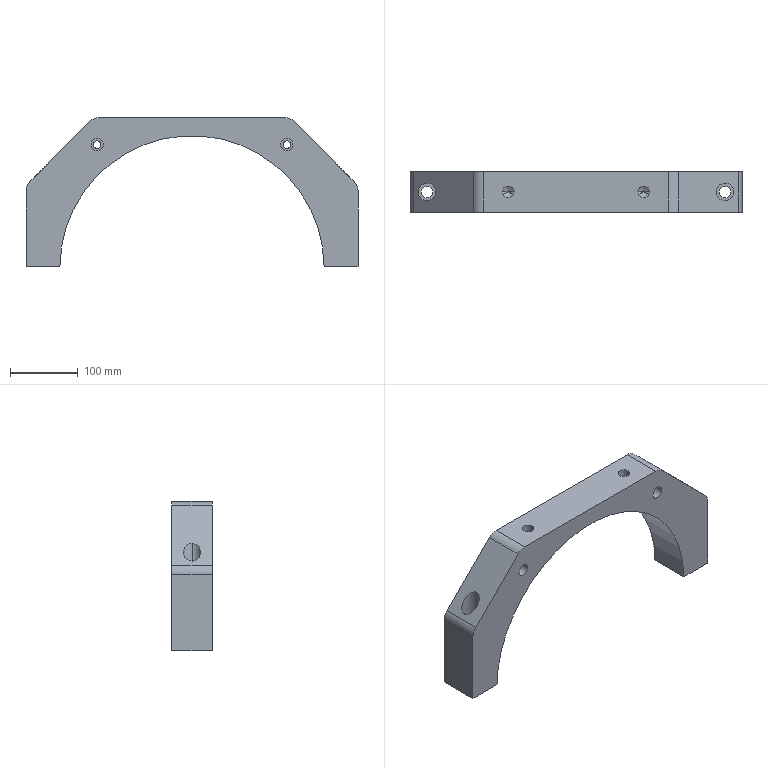Part | NX | features BREP 1 | 1 solid | 48 faces | box 490 x 60 x 220 mm | volume 2146517 mm3 | cylinder 29 | plane 15 | cone 4 | commonest cylinder face diameters 11 x4 17 x4 17.294 x4 18 x4 26 x4 30 x4
STEP:
#1=CARTESIAN_POINT('',(245.,30.,0.));
#2=VERTEX_POINT('',#1);
#3=CARTESIAN_POINT('',(245.,-30.,0.));
#4=VERTEX_POINT('',#3);
#5=CARTESIAN_POINT('',(245.,30.,0.));
#6=DIRECTION('',(0.,-1.,0.));
#7=VECTOR('',#6,1000.);
#8=LINE('',#5,#7);
#9=EDGE_CURVE('',#2,#4,#8,.T.);
#10=ORIENTED_EDGE('',*,*,#9,.F.);
#11=CARTESIAN_POINT('',(245.,30.,111.716));
#12=VERTEX_POINT('',#11);
#13=CARTESIAN_POINT('',(245.,30.,0.));
#14=DIRECTION('',(0.,0.,1.));
#15=VECTOR('',#14,1000.);
#16=LINE('',#13,#15);
#17=EDGE_CURVE('',#2,#12,#16,.T.);
#18=ORIENTED_EDGE('',*,*,#17,.T.);
#19=CARTESIAN_POINT('',(245.,-30.,111.716));
#20=VERTEX_POINT('',#19);
#21=CARTESIAN_POINT('',(245.,-30.,111.716));
#22=DIRECTION('',(0.,1.,0.));
#23=VECTOR('',#22,1000.);
#24=LINE('',#21,#23);
#25=EDGE_CURVE('',#20,#12,#24,.T.);
#26=ORIENTED_EDGE('',*,*,#25,.F.);
#27=CARTESIAN_POINT('',(245.,-30.,0.));
#28=DIRECTION('',(0.,0.,1.));
#29=VECTOR('',#28,1000.);
#30=LINE('',#27,#29);
#31=EDGE_CURVE('',#4,#20,#30,.T.);
#32=ORIENTED_EDGE('',*,*,#31,.F.);
#33=EDGE_LOOP('',(#10,#18,#26,#32));
#34=FACE_BOUND('',#33,.T.);
#35=CARTESIAN_POINT('',(245.,0.,220.));
#36=DIRECTION('',(1.,0.,0.));
#37=DIRECTION('',(0.,1.,0.));
#38=AXIS2_PLACEMENT_3D('',#35,#36,#37);
#39=PLANE('',#38);
#40=ADVANCED_FACE('',(#34),#39,.T.);
#41=CARTESIAN_POINT('',(239.142,-30.,125.858));
#42=VERTEX_POINT('',#41);
#43=CARTESIAN_POINT('',(150.858,-30.,214.142));
#44=VERTEX_POINT('',#43);
#45=CARTESIAN_POINT('',(239.142,-30.,125.858));
#46=DIRECTION('',(-0.7071,0.,0.7071));
#47=VECTOR('',#46,1000.);
#48=LINE('',#45,#47);
#49=EDGE_CURVE('',#42,#44,#48,.T.);
#50=ORIENTED_EDGE('',*,*,#49,.T.);
#51=CARTESIAN_POINT('',(136.716,-30.,220.));
#52=VERTEX_POINT('',#51);
#53=CARTESIAN_POINT('',(136.716,-30.,200.));
#54=DIRECTION('',(0.,-1.,0.));
#55=DIRECTION('',(0.7071,0.,0.7071));
#56=AXIS2_PLACEMENT_3D('',#53,#54,#55);
#57=CIRCLE('',#56,20.);
#58=EDGE_CURVE('',#44,#52,#57,.T.);
#59=ORIENTED_EDGE('',*,*,#58,.T.);
#60=CARTESIAN_POINT('',(-136.716,-30.,220.));
#61=VERTEX_POINT('',#60);
#62=CARTESIAN_POINT('',(136.716,-30.,220.));
#63=DIRECTION('',(-1.,0.,0.));
#64=VECTOR('',#63,1000.);
#65=LINE('',#62,#64);
#66=EDGE_CURVE('',#52,#61,#65,.T.);
#67=ORIENTED_EDGE('',*,*,#66,.T.);
#68=CARTESIAN_POINT('',(-150.858,-30.,214.142));
#69=VERTEX_POINT('',#68);
#70=CARTESIAN_POINT('',(-136.716,-30.,200.));
#71=DIRECTION('',(0.,-1.,0.));
#72=DIRECTION('',(0.,0.,1.));
#73=AXIS2_PLACEMENT_3D('',#70,#71,#72);
#74=CIRCLE('',#73,20.);
#75=EDGE_CURVE('',#61,#69,#74,.T.);
#76=ORIENTED_EDGE('',*,*,#75,.T.);
#77=CARTESIAN_POINT('',(-239.142,-30.,125.858));
#78=VERTEX_POINT('',#77);
#79=CARTESIAN_POINT('',(-150.858,-30.,214.142));
#80=DIRECTION('',(-0.7071,0.,-0.7071));
#81=VECTOR('',#80,1000.);
#82=LINE('',#79,#81);
#83=EDGE_CURVE('',#69,#78,#82,.T.);
#84=ORIENTED_EDGE('',*,*,#83,.T.);
#85=CARTESIAN_POINT('',(-245.,-30.,111.716));
#86=VERTEX_POINT('',#85);
#87=CARTESIAN_POINT('',(-225.,-30.,111.716));
#88=DIRECTION('',(0.,-1.,0.));
#89=DIRECTION('',(-0.7071,0.,0.7071));
#90=AXIS2_PLACEMENT_3D('',#87,#88,#89);
#91=CIRCLE('',#90,20.);
#92=EDGE_CURVE('',#78,#86,#91,.T.);
#93=ORIENTED_EDGE('',*,*,#92,.T.);
#94=CARTESIAN_POINT('',(-245.,-30.,0.));
#95=VERTEX_POINT('',#94);
#96=CARTESIAN_POINT('',(-245.,-30.,111.716));
#97=DIRECTION('',(0.,0.,-1.));
#98=VECTOR('',#97,1000.);
#99=LINE('',#96,#98);
#100=EDGE_CURVE('',#86,#95,#99,.T.);
#101=ORIENTED_EDGE('',*,*,#100,.T.);
#102=CARTESIAN_POINT('',(-194.99,-30.,0.));
#103=VERTEX_POINT('',#102);
#104=CARTESIAN_POINT('',(-245.,-30.,0.));
#105=DIRECTION('',(1.,0.,0.));
#106=VECTOR('',#105,1000.);
#107=LINE('',#104,#106);
#108=EDGE_CURVE('',#95,#103,#107,.T.);
#109=ORIENTED_EDGE('',*,*,#108,.T.);
#110=CARTESIAN_POINT('',(194.99,-30.,0.));
#111=VERTEX_POINT('',#110);
#112=CARTESIAN_POINT('',(0.,-30.,-2.));
#113=DIRECTION('',(0.,1.,0.));
#114=DIRECTION('',(-0.9999,0.,0.01026));
#115=AXIS2_PLACEMENT_3D('',#112,#113,#114);
#116=CIRCLE('',#115,195.);
#117=EDGE_CURVE('',#103,#111,#116,.T.);
#118=ORIENTED_EDGE('',*,*,#117,.T.);
#119=CARTESIAN_POINT('',(194.99,-30.,0.));
#120=DIRECTION('',(1.,0.,0.));
#121=VECTOR('',#120,1000.);
#122=LINE('',#119,#121);
#123=EDGE_CURVE('',#111,#4,#122,.T.);
#124=ORIENTED_EDGE('',*,*,#123,.T.);
#125=ORIENTED_EDGE('',*,*,#31,.T.);
#126=CARTESIAN_POINT('',(225.,-30.,111.716));
#127=DIRECTION('',(0.,-1.,0.));
#128=DIRECTION('',(1.,0.,0.));
#129=AXIS2_PLACEMENT_3D('',#126,#127,#128);
#130=CIRCLE('',#129,20.);
#131=EDGE_CURVE('',#20,#42,#130,.T.);
#132=ORIENTED_EDGE('',*,*,#131,.T.);
#133=EDGE_LOOP('',(#50,#59,#67,#76,#84,#93,#101,#109,#118,#124,#125,#132));
#134=FACE_BOUND('',#133,.T.);
#135=CARTESIAN_POINT('',(131.,-30.,180.));
#136=VERTEX_POINT('',#135);
#137=CARTESIAN_POINT('',(149.,-30.,180.));
#138=VERTEX_POINT('',#137);
#139=CARTESIAN_POINT('',(140.,-30.,180.));
#140=DIRECTION('',(0.,1.,0.));
#141=DIRECTION('',(-1.,0.,0.));
#142=AXIS2_PLACEMENT_3D('',#139,#140,#141);
#143=CIRCLE('',#142,9.);
#144=EDGE_CURVE('',#136,#138,#143,.T.);
#145=ORIENTED_EDGE('',*,*,#144,.T.);
#146=CARTESIAN_POINT('',(140.,-30.,180.));
#147=DIRECTION('',(0.,1.,0.));
#148=DIRECTION('',(1.,0.,0.));
#149=AXIS2_PLACEMENT_3D('',#146,#147,#148);
#150=CIRCLE('',#149,9.);
#151=EDGE_CURVE('',#138,#136,#150,.T.);
#152=ORIENTED_EDGE('',*,*,#151,.T.);
#153=EDGE_LOOP('',(#145,#152));
#154=FACE_BOUND('',#153,.T.);
#155=CARTESIAN_POINT('',(-131.,-30.,180.));
#156=VERTEX_POINT('',#155);
#157=CARTESIAN_POINT('',(-149.,-30.,180.));
#158=VERTEX_POINT('',#157);
#159=CARTESIAN_POINT('',(-140.,-30.,180.));
#160=DIRECTION('',(0.,1.,0.));
#161=DIRECTION('',(1.,0.,0.));
#162=AXIS2_PLACEMENT_3D('',#159,#160,#161);
#163=CIRCLE('',#162,9.);
#164=EDGE_CURVE('',#156,#158,#163,.T.);
#165=ORIENTED_EDGE('',*,*,#164,.T.);
#166=CARTESIAN_POINT('',(-140.,-30.,180.));
#167=DIRECTION('',(0.,1.,0.));
#168=DIRECTION('',(-1.,0.,0.));
#169=AXIS2_PLACEMENT_3D('',#166,#167,#168);
#170=CIRCLE('',#169,9.);
#171=EDGE_CURVE('',#158,#156,#170,.T.);
#172=ORIENTED_EDGE('',*,*,#171,.T.);
#173=EDGE_LOOP('',(#165,#172));
#174=FACE_BOUND('',#173,.T.);
#175=CARTESIAN_POINT('',(0.,-30.,0.));
#176=DIRECTION('',(0.,1.,0.));
#177=DIRECTION('',(1.,0.,0.));
#178=AXIS2_PLACEMENT_3D('',#175,#176,#177);
#179=PLANE('',#178);
#180=ADVANCED_FACE('',(#134,#154,#174),#179,.F.);
#181=CARTESIAN_POINT('',(239.142,30.,125.858));
#182=VERTEX_POINT('',#181);
#183=CARTESIAN_POINT('',(239.142,30.,125.858));
#184=DIRECTION('',(0.,-1.,0.));
#185=VECTOR('',#184,1000.);
#186=LINE('',#183,#185);
#187=EDGE_CURVE('',#182,#42,#186,.T.);
#188=ORIENTED_EDGE('',*,*,#187,.T.);
#189=ORIENTED_EDGE('',*,*,#131,.F.);
#190=ORIENTED_EDGE('',*,*,#25,.T.);
#191=CARTESIAN_POINT('',(225.,30.,111.716));
#192=DIRECTION('',(0.,1.,0.));
#193=DIRECTION('',(0.7071,0.,0.7071));
#194=AXIS2_PLACEMENT_3D('',#191,#192,#193);
#195=CIRCLE('',#194,20.);
#196=EDGE_CURVE('',#182,#12,#195,.T.);
#197=ORIENTED_EDGE('',*,*,#196,.F.);
#198=EDGE_LOOP('',(#188,#189,#190,#197));
#199=FACE_BOUND('',#198,.T.);
#200=CARTESIAN_POINT('',(225.,0.,111.716));
#201=DIRECTION('',(0.,1.,0.));
#202=DIRECTION('',(0.7071,0.,0.7071));
#203=AXIS2_PLACEMENT_3D('',#200,#201,#202);
#204=CYLINDRICAL_SURFACE('',#203,20.);
#205=ADVANCED_FACE('',(#199),#204,.T.);
#206=CARTESIAN_POINT('',(194.99,30.,0.));
#207=VERTEX_POINT('',#206);
#208=CARTESIAN_POINT('',(194.99,30.,0.));
#209=DIRECTION('',(1.,0.,0.));
#210=VECTOR('',#209,1000.);
#211=LINE('',#208,#210);
#212=EDGE_CURVE('',#207,#2,#211,.T.);
#213=ORIENTED_EDGE('',*,*,#212,.F.);
#214=CARTESIAN_POINT('',(-194.99,30.,0.));
#215=VERTEX_POINT('',#214);
#216=CARTESIAN_POINT('',(0.,30.,-2.));
#217=DIRECTION('',(0.,-1.,0.));
#218=DIRECTION('',(0.9999,0.,0.01026));
#219=AXIS2_PLACEMENT_3D('',#216,#217,#218);
#220=CIRCLE('',#219,195.);
#221=EDGE_CURVE('',#207,#215,#220,.T.);
#222=ORIENTED_EDGE('',*,*,#221,.T.);
#223=CARTESIAN_POINT('',(-245.,30.,0.));
#224=VERTEX_POINT('',#223);
#225=CARTESIAN_POINT('',(-245.,30.,0.));
#226=DIRECTION('',(1.,0.,0.));
#227=VECTOR('',#226,1000.);
#228=LINE('',#225,#227);
#229=EDGE_CURVE('',#224,#215,#228,.T.);
#230=ORIENTED_EDGE('',*,*,#229,.F.);
#231=CARTESIAN_POINT('',(-245.,30.,111.716));
#232=VERTEX_POINT('',#231);
#233=CARTESIAN_POINT('',(-245.,30.,111.716));
#234=DIRECTION('',(0.,0.,-1.));
#235=VECTOR('',#234,1000.);
#236=LINE('',#233,#235);
#237=EDGE_CURVE('',#232,#224,#236,.T.);
#238=ORIENTED_EDGE('',*,*,#237,.F.);
#239=CARTESIAN_POINT('',(-239.142,30.,125.858));
#240=VERTEX_POINT('',#239);
#241=CARTESIAN_POINT('',(-225.,30.,111.716));
#242=DIRECTION('',(0.,1.,0.));
#243=DIRECTION('',(-1.,0.,0.));
#244=AXIS2_PLACEMENT_3D('',#241,#242,#243);
#245=CIRCLE('',#244,20.);
#246=EDGE_CURVE('',#232,#240,#245,.T.);
#247=ORIENTED_EDGE('',*,*,#246,.T.);
#248=CARTESIAN_POINT('',(-150.858,30.,214.142));
#249=VERTEX_POINT('',#248);
#250=CARTESIAN_POINT('',(-239.142,30.,125.858));
#251=DIRECTION('',(0.7071,0.,0.7071));
#252=VECTOR('',#251,1000.);
#253=LINE('',#250,#252);
#254=EDGE_CURVE('',#240,#249,#253,.T.);
#255=ORIENTED_EDGE('',*,*,#254,.T.);
#256=CARTESIAN_POINT('',(-136.716,30.,220.));
#257=VERTEX_POINT('',#256);
#258=CARTESIAN_POINT('',(-136.716,30.,200.));
#259=DIRECTION('',(0.,1.,0.));
#260=DIRECTION('',(-0.7071,0.,0.7071));
#261=AXIS2_PLACEMENT_3D('',#258,#259,#260);
#262=CIRCLE('',#261,20.);
#263=EDGE_CURVE('',#249,#257,#262,.T.);
#264=ORIENTED_EDGE('',*,*,#263,.T.);
#265=CARTESIAN_POINT('',(136.716,30.,220.));
#266=VERTEX_POINT('',#265);
#267=CARTESIAN_POINT('',(136.716,30.,220.));
#268=DIRECTION('',(-1.,0.,0.));
#269=VECTOR('',#268,1000.);
#270=LINE('',#267,#269);
#271=EDGE_CURVE('',#266,#257,#270,.T.);
#272=ORIENTED_EDGE('',*,*,#271,.F.);
#273=CARTESIAN_POINT('',(150.858,30.,214.142));
#274=VERTEX_POINT('',#273);
#275=CARTESIAN_POINT('',(136.716,30.,200.));
#276=DIRECTION('',(0.,1.,0.));
#277=DIRECTION('',(0.,0.,1.));
#278=AXIS2_PLACEMENT_3D('',#275,#276,#277);
#279=CIRCLE('',#278,20.);
#280=EDGE_CURVE('',#266,#274,#279,.T.);
#281=ORIENTED_EDGE('',*,*,#280,.T.);
#282=CARTESIAN_POINT('',(150.858,30.,214.142));
#283=DIRECTION('',(0.7071,0.,-0.7071));
#284=VECTOR('',#283,1000.);
#285=LINE('',#282,#284);
#286=EDGE_CURVE('',#274,#182,#285,.T.);
#287=ORIENTED_EDGE('',*,*,#286,.T.);
#288=ORIENTED_EDGE('',*,*,#196,.T.);
#289=ORIENTED_EDGE('',*,*,#17,.F.);
#290=EDGE_LOOP('',(#213,#222,#230,#238,#247,#255,#264,#272,#281,#287,#288,#289));
#291=FACE_BOUND('',#290,.T.);
#292=CARTESIAN_POINT('',(125.,30.,180.));
#293=VERTEX_POINT('',#292);
#294=CARTESIAN_POINT('',(155.,30.,180.));
#295=VERTEX_POINT('',#294);
#296=CARTESIAN_POINT('',(140.,30.,180.));
#297=DIRECTION('',(0.,-1.,0.));
#298=DIRECTION('',(-1.,0.,0.));
#299=AXIS2_PLACEMENT_3D('',#296,#297,#298);
#300=CIRCLE('',#299,15.);
#301=EDGE_CURVE('',#293,#295,#300,.T.);
#302=ORIENTED_EDGE('',*,*,#301,.T.);
#303=CARTESIAN_POINT('',(140.,30.,180.));
#304=DIRECTION('',(0.,-1.,0.));
#305=DIRECTION('',(1.,0.,0.));
#306=AXIS2_PLACEMENT_3D('',#303,#304,#305);
#307=CIRCLE('',#306,15.);
#308=EDGE_CURVE('',#295,#293,#307,.T.);
#309=ORIENTED_EDGE('',*,*,#308,.T.);
#310=EDGE_LOOP('',(#302,#309));
#311=FACE_BOUND('',#310,.T.);
#312=CARTESIAN_POINT('',(-125.,30.,180.));
#313=VERTEX_POINT('',#312);
#314=CARTESIAN_POINT('',(-155.,30.,180.));
#315=VERTEX_POINT('',#314);
#316=CARTESIAN_POINT('',(-140.,30.,180.));
#317=DIRECTION('',(0.,-1.,0.));
#318=DIRECTION('',(1.,0.,0.));
#319=AXIS2_PLACEMENT_3D('',#316,#317,#318);
#320=CIRCLE('',#319,15.);
#321=EDGE_CURVE('',#313,#315,#320,.T.);
#322=ORIENTED_EDGE('',*,*,#321,.T.);
#323=CARTESIAN_POINT('',(-140.,30.,180.));
#324=DIRECTION('',(0.,-1.,0.));
#325=DIRECTION('',(-1.,0.,0.));
#326=AXIS2_PLACEMENT_3D('',#323,#324,#325);
#327=CIRCLE('',#326,15.);
#328=EDGE_CURVE('',#315,#313,#327,.T.);
#329=ORIENTED_EDGE('',*,*,#328,.T.);
#330=EDGE_LOOP('',(#322,#329));
#331=FACE_BOUND('',#330,.T.);
#332=CARTESIAN_POINT('',(0.,30.,0.));
#333=DIRECTION('',(0.,1.,0.));
#334=DIRECTION('',(1.,0.,0.));
#335=AXIS2_PLACEMENT_3D('',#332,#333,#334);
#336=PLANE('',#335);
#337=ADVANCED_FACE('',(#291,#311,#331),#336,.T.);
#338=CARTESIAN_POINT('',(150.858,-30.,214.142));
#339=DIRECTION('',(0.,1.,0.));
#340=VECTOR('',#339,1000.);
#341=LINE('',#338,#340);
#342=EDGE_CURVE('',#44,#274,#341,.T.);
#343=ORIENTED_EDGE('',*,*,#342,.F.);
#344=ORIENTED_EDGE('',*,*,#49,.F.);
#345=ORIENTED_EDGE('',*,*,#187,.F.);
#346=ORIENTED_EDGE('',*,*,#286,.F.);
#347=EDGE_LOOP('',(#343,#344,#345,#346));
#348=FACE_BOUND('',#347,.T.);
#349=CARTESIAN_POINT('',(233.,0.,132.));
#350=VERTEX_POINT('',#349);
#351=CARTESIAN_POINT('',(207.,0.,158.));
#352=VERTEX_POINT('',#351);
#353=CARTESIAN_POINT('',(233.,0.,132.));
#354=CARTESIAN_POINT('',(233.,-0.757,132.));
#355=CARTESIAN_POINT('',(232.865,-2.26,132.135));
#356=CARTESIAN_POINT('',(232.31,-4.393,132.69));
#357=CARTESIAN_POINT('',(231.246,-6.675,133.754));
#358=CARTESIAN_POINT('',(230.126,-8.23,134.874));
#359=CARTESIAN_POINT('',(228.875,-9.533,136.125));
#360=CARTESIAN_POINT('',(227.886,-10.366,137.114));
#361=CARTESIAN_POINT('',(226.8,-11.107,138.2));
#362=CARTESIAN_POINT('',(225.679,-11.722,139.321));
#363=CARTESIAN_POINT('',(224.317,-12.294,140.683));
#364=CARTESIAN_POINT('',(222.526,-12.816,142.474));
#365=CARTESIAN_POINT('',(220.151,-13.102,144.849));
#366=CARTESIAN_POINT('',(217.735,-12.866,147.265));
#367=CARTESIAN_POINT('',(215.917,-12.373,149.083));
#368=CARTESIAN_POINT('',(214.533,-11.822,150.467));
#369=CARTESIAN_POINT('',(213.375,-11.214,151.625));
#370=CARTESIAN_POINT('',(212.257,-10.476,152.743));
#371=CARTESIAN_POINT('',(211.239,-9.64,153.761));
#372=CARTESIAN_POINT('',(209.95,-8.325,155.05));
#373=CARTESIAN_POINT('',(208.797,-6.751,156.203));
#374=CARTESIAN_POINT('',(207.701,-4.432,157.299));
#375=CARTESIAN_POINT('',(207.138,-2.286,157.862));
#376=CARTESIAN_POINT('',(207.,-0.7657,158.));
#377=CARTESIAN_POINT('',(207.,0.,158.));
#378=B_SPLINE_CURVE_WITH_KNOTS('',3,(#353,#354,#355,#356,#357,#358,#359,#360,#361,#362,#363,#364,#365,#366,#367,#368,#369,#370,#371,#372,#373,#374,#375,#376,#377),.UNSPECIFIED.,.F.,.F.,(4,1,1,1,1,1,1,1,1,1,1,1,1,1,1,1,1,1,1,1,1,1,4),(0.,0.0625,0.125,0.1875,0.25,0.2812,0.3125,0.3438,0.375,0.4062,0.4375,0.5,0.5625,0.5938,0.625,0.6562,0.6875,0.7188,0.75,0.8125,0.875,0.9375,1.),.UNSPECIFIED.);
#379=EDGE_CURVE('',#350,#352,#378,.T.);
#380=ORIENTED_EDGE('',*,*,#379,.T.);
#381=CARTESIAN_POINT('',(207.,0.,158.));
#382=CARTESIAN_POINT('',(207.,0.7586,158.));
#383=CARTESIAN_POINT('',(207.136,2.265,157.864));
#384=CARTESIAN_POINT('',(207.693,4.402,157.307));
#385=CARTESIAN_POINT('',(208.762,6.688,156.238));
#386=CARTESIAN_POINT('',(209.885,8.244,155.115));
#387=CARTESIAN_POINT('',(211.142,9.549,153.858));
#388=CARTESIAN_POINT('',(212.135,10.382,152.865));
#389=CARTESIAN_POINT('',(213.226,11.123,151.774));
#390=CARTESIAN_POINT('',(214.352,11.736,150.648));
#391=CARTESIAN_POINT('',(215.717,12.306,149.283));
#392=CARTESIAN_POINT('',(217.512,12.823,147.488));
#393=CARTESIAN_POINT('',(219.895,13.103,145.105));
#394=CARTESIAN_POINT('',(222.304,12.859,142.696));
#395=CARTESIAN_POINT('',(224.118,12.362,140.882));
#396=CARTESIAN_POINT('',(225.5,11.807,139.5));
#397=CARTESIAN_POINT('',(226.652,11.198,138.348));
#398=CARTESIAN_POINT('',(227.764,10.46,137.236));
#399=CARTESIAN_POINT('',(228.778,9.625,136.222));
#400=CARTESIAN_POINT('',(230.061,8.311,134.939));
#401=CARTESIAN_POINT('',(231.207,6.743,133.793));
#402=CARTESIAN_POINT('',(232.299,4.43,132.701));
#403=CARTESIAN_POINT('',(232.862,2.284,132.138));
#404=CARTESIAN_POINT('',(233.,0.765,132.));
#405=CARTESIAN_POINT('',(233.,0.,132.));
#406=B_SPLINE_CURVE_WITH_KNOTS('',3,(#381,#382,#383,#384,#385,#386,#387,#388,#389,#390,#391,#392,#393,#394,#395,#396,#397,#398,#399,#400,#401,#402,#403,#404,#405),.UNSPECIFIED.,.F.,.F.,(4,1,1,1,1,1,1,1,1,1,1,1,1,1,1,1,1,1,1,1,1,1,4),(0.,0.0625,0.125,0.1875,0.25,0.2812,0.3125,0.3438,0.375,0.4062,0.4375,0.5,0.5625,0.5938,0.625,0.6562,0.6875,0.7188,0.75,0.8125,0.875,0.9375,1.),.UNSPECIFIED.);
#407=EDGE_CURVE('',#352,#350,#406,.T.);
#408=ORIENTED_EDGE('',*,*,#407,.T.);
#409=EDGE_LOOP('',(#380,#408));
#410=FACE_BOUND('',#409,.T.);
#411=CARTESIAN_POINT('',(245.,0.,120.));
#412=DIRECTION('',(0.7071,0.,0.7071));
#413=DIRECTION('',(0.,-1.,0.));
#414=AXIS2_PLACEMENT_3D('',#411,#412,#413);
#415=PLANE('',#414);
#416=ADVANCED_FACE('',(#348,#410),#415,.T.);
#417=CARTESIAN_POINT('',(136.716,30.,220.));
#418=DIRECTION('',(0.,-1.,0.));
#419=VECTOR('',#418,1000.);
#420=LINE('',#417,#419);
#421=EDGE_CURVE('',#266,#52,#420,.T.);
#422=ORIENTED_EDGE('',*,*,#421,.T.);
#423=ORIENTED_EDGE('',*,*,#58,.F.);
#424=ORIENTED_EDGE('',*,*,#342,.T.);
#425=ORIENTED_EDGE('',*,*,#280,.F.);
#426=EDGE_LOOP('',(#422,#423,#424,#425));
#427=FACE_BOUND('',#426,.T.);
#428=CARTESIAN_POINT('',(136.716,0.,200.));
#429=DIRECTION('',(0.,1.,0.));
#430=DIRECTION('',(0.,0.,1.));
#431=AXIS2_PLACEMENT_3D('',#428,#429,#430);
#432=CYLINDRICAL_SURFACE('',#431,20.);
#433=ADVANCED_FACE('',(#427),#432,.T.);
#434=ORIENTED_EDGE('',*,*,#271,.T.);
#435=CARTESIAN_POINT('',(-136.716,-30.,220.));
#436=DIRECTION('',(0.,1.,0.));
#437=VECTOR('',#436,1000.);
#438=LINE('',#435,#437);
#439=EDGE_CURVE('',#61,#257,#438,.T.);
#440=ORIENTED_EDGE('',*,*,#439,.F.);
#441=ORIENTED_EDGE('',*,*,#66,.F.);
#442=ORIENTED_EDGE('',*,*,#421,.F.);
#443=EDGE_LOOP('',(#434,#440,#441,#442));
#444=FACE_BOUND('',#443,.T.);
#445=CARTESIAN_POINT('',(-91.353,0.,220.));
#446=VERTEX_POINT('',#445);
#447=CARTESIAN_POINT('',(-108.647,0.,220.));
#448=VERTEX_POINT('',#447);
#449=CARTESIAN_POINT('',(-100.,0.,220.));
#450=DIRECTION('',(0.,0.,-1.));
#451=DIRECTION('',(1.,0.,0.));
#452=AXIS2_PLACEMENT_3D('',#449,#450,#451);
#453=CIRCLE('',#452,8.647);
#454=EDGE_CURVE('',#446,#448,#453,.T.);
#455=ORIENTED_EDGE('',*,*,#454,.T.);
#456=CARTESIAN_POINT('',(-100.,0.,220.));
#457=DIRECTION('',(0.,0.,-1.));
#458=DIRECTION('',(-1.,0.,0.));
#459=AXIS2_PLACEMENT_3D('',#456,#457,#458);
#460=CIRCLE('',#459,8.647);
#461=EDGE_CURVE('',#448,#446,#460,.T.);
#462=ORIENTED_EDGE('',*,*,#461,.T.);
#463=EDGE_LOOP('',(#455,#462));
#464=FACE_BOUND('',#463,.T.);
#465=CARTESIAN_POINT('',(108.647,0.,220.));
#466=VERTEX_POINT('',#465);
#467=CARTESIAN_POINT('',(91.353,0.,220.));
#468=VERTEX_POINT('',#467);
#469=CARTESIAN_POINT('',(100.,0.,220.));
#470=DIRECTION('',(0.,0.,-1.));
#471=DIRECTION('',(1.,0.,0.));
#472=AXIS2_PLACEMENT_3D('',#469,#470,#471);
#473=CIRCLE('',#472,8.647);
#474=EDGE_CURVE('',#466,#468,#473,.T.);
#475=ORIENTED_EDGE('',*,*,#474,.T.);
#476=CARTESIAN_POINT('',(100.,0.,220.));
#477=DIRECTION('',(0.,0.,-1.));
#478=DIRECTION('',(-1.,0.,0.));
#479=AXIS2_PLACEMENT_3D('',#476,#477,#478);
#480=CIRCLE('',#479,8.647);
#481=EDGE_CURVE('',#468,#466,#480,.T.);
#482=ORIENTED_EDGE('',*,*,#481,.T.);
#483=EDGE_LOOP('',(#475,#482));
#484=FACE_BOUND('',#483,.T.);
#485=CARTESIAN_POINT('',(245.,0.,220.));
#486=DIRECTION('',(0.,0.,-1.));
#487=DIRECTION('',(0.,-1.,0.));
#488=AXIS2_PLACEMENT_3D('',#485,#486,#487);
#489=PLANE('',#488);
#490=ADVANCED_FACE('',(#444,#464,#484),#489,.F.);
#491=CARTESIAN_POINT('',(-150.858,30.,214.142));
#492=DIRECTION('',(0.,-1.,0.));
#493=VECTOR('',#492,1000.);
#494=LINE('',#491,#493);
#495=EDGE_CURVE('',#249,#69,#494,.T.);
#496=ORIENTED_EDGE('',*,*,#495,.T.);
#497=ORIENTED_EDGE('',*,*,#75,.F.);
#498=ORIENTED_EDGE('',*,*,#439,.T.);
#499=ORIENTED_EDGE('',*,*,#263,.F.);
#500=EDGE_LOOP('',(#496,#497,#498,#499));
#501=FACE_BOUND('',#500,.T.);
#502=CARTESIAN_POINT('',(-136.716,0.,200.));
#503=DIRECTION('',(0.,1.,0.));
#504=DIRECTION('',(-0.7071,0.,0.7071));
#505=AXIS2_PLACEMENT_3D('',#502,#503,#504);
#506=CYLINDRICAL_SURFACE('',#505,20.);
#507=ADVANCED_FACE('',(#501),#506,.T.);
#508=ORIENTED_EDGE('',*,*,#83,.F.);
#509=ORIENTED_EDGE('',*,*,#495,.F.);
#510=ORIENTED_EDGE('',*,*,#254,.F.);
#511=CARTESIAN_POINT('',(-239.142,-30.,125.858));
#512=DIRECTION('',(0.,1.,0.));
#513=VECTOR('',#512,1000.);
#514=LINE('',#511,#513);
#515=EDGE_CURVE('',#78,#240,#514,.T.);
#516=ORIENTED_EDGE('',*,*,#515,.F.);
#517=EDGE_LOOP('',(#508,#509,#510,#516));
#518=FACE_BOUND('',#517,.T.);
#519=CARTESIAN_POINT('',(-233.,0.,132.));
#520=VERTEX_POINT('',#519);
#521=CARTESIAN_POINT('',(-207.,0.,158.));
#522=VERTEX_POINT('',#521);
#523=CARTESIAN_POINT('',(-233.,0.,132.));
#524=CARTESIAN_POINT('',(-233.,0.757,132.));
#525=CARTESIAN_POINT('',(-232.865,2.26,132.135));
#526=CARTESIAN_POINT('',(-232.31,4.393,132.69));
#527=CARTESIAN_POINT('',(-231.246,6.675,133.754));
#528=CARTESIAN_POINT('',(-230.126,8.23,134.874));
#529=CARTESIAN_POINT('',(-228.875,9.533,136.125));
#530=CARTESIAN_POINT('',(-227.886,10.366,137.114));
#531=CARTESIAN_POINT('',(-226.8,11.107,138.2));
#532=CARTESIAN_POINT('',(-225.679,11.722,139.321));
#533=CARTESIAN_POINT('',(-224.317,12.294,140.683));
#534=CARTESIAN_POINT('',(-222.526,12.816,142.474));
#535=CARTESIAN_POINT('',(-220.151,13.102,144.849));
#536=CARTESIAN_POINT('',(-217.735,12.866,147.265));
#537=CARTESIAN_POINT('',(-215.917,12.373,149.083));
#538=CARTESIAN_POINT('',(-214.533,11.822,150.467));
#539=CARTESIAN_POINT('',(-213.375,11.214,151.625));
#540=CARTESIAN_POINT('',(-212.257,10.476,152.743));
#541=CARTESIAN_POINT('',(-211.239,9.64,153.761));
#542=CARTESIAN_POINT('',(-209.95,8.325,155.05));
#543=CARTESIAN_POINT('',(-208.797,6.751,156.203));
#544=CARTESIAN_POINT('',(-207.701,4.432,157.299));
#545=CARTESIAN_POINT('',(-207.138,2.286,157.862));
#546=CARTESIAN_POINT('',(-207.,0.7657,158.));
#547=CARTESIAN_POINT('',(-207.,0.,158.));
#548=B_SPLINE_CURVE_WITH_KNOTS('',3,(#523,#524,#525,#526,#527,#528,#529,#530,#531,#532,#533,#534,#535,#536,#537,#538,#539,#540,#541,#542,#543,#544,#545,#546,#547),.UNSPECIFIED.,.F.,.F.,(4,1,1,1,1,1,1,1,1,1,1,1,1,1,1,1,1,1,1,1,1,1,4),(0.,0.0625,0.125,0.1875,0.25,0.2812,0.3125,0.3438,0.375,0.4062,0.4375,0.5,0.5625,0.5938,0.625,0.6562,0.6875,0.7188,0.75,0.8125,0.875,0.9375,1.),.UNSPECIFIED.);
#549=EDGE_CURVE('',#520,#522,#548,.T.);
#550=ORIENTED_EDGE('',*,*,#549,.T.);
#551=CARTESIAN_POINT('',(-207.,0.,158.));
#552=CARTESIAN_POINT('',(-207.,-0.7586,158.));
#553=CARTESIAN_POINT('',(-207.136,-2.265,157.864));
#554=CARTESIAN_POINT('',(-207.693,-4.402,157.307));
#555=CARTESIAN_POINT('',(-208.762,-6.688,156.238));
#556=CARTESIAN_POINT('',(-209.885,-8.244,155.115));
#557=CARTESIAN_POINT('',(-211.142,-9.549,153.858));
#558=CARTESIAN_POINT('',(-212.135,-10.382,152.865));
#559=CARTESIAN_POINT('',(-213.226,-11.123,151.774));
#560=CARTESIAN_POINT('',(-214.352,-11.736,150.648));
#561=CARTESIAN_POINT('',(-215.717,-12.306,149.283));
#562=CARTESIAN_POINT('',(-217.512,-12.823,147.488));
#563=CARTESIAN_POINT('',(-219.895,-13.103,145.105));
#564=CARTESIAN_POINT('',(-222.304,-12.859,142.696));
#565=CARTESIAN_POINT('',(-224.118,-12.362,140.882));
#566=CARTESIAN_POINT('',(-225.5,-11.807,139.5));
#567=CARTESIAN_POINT('',(-226.652,-11.198,138.348));
#568=CARTESIAN_POINT('',(-227.764,-10.46,137.236));
#569=CARTESIAN_POINT('',(-228.778,-9.625,136.222));
#570=CARTESIAN_POINT('',(-230.061,-8.311,134.939));
#571=CARTESIAN_POINT('',(-231.207,-6.743,133.793));
#572=CARTESIAN_POINT('',(-232.299,-4.43,132.701));
#573=CARTESIAN_POINT('',(-232.862,-2.284,132.138));
#574=CARTESIAN_POINT('',(-233.,-0.765,132.));
#575=CARTESIAN_POINT('',(-233.,0.,132.));
#576=B_SPLINE_CURVE_WITH_KNOTS('',3,(#551,#552,#553,#554,#555,#556,#557,#558,#559,#560,#561,#562,#563,#564,#565,#566,#567,#568,#569,#570,#571,#572,#573,#574,#575),.UNSPECIFIED.,.F.,.F.,(4,1,1,1,1,1,1,1,1,1,1,1,1,1,1,1,1,1,1,1,1,1,4),(0.,0.0625,0.125,0.1875,0.25,0.2812,0.3125,0.3438,0.375,0.4062,0.4375,0.5,0.5625,0.5938,0.625,0.6562,0.6875,0.7188,0.75,0.8125,0.875,0.9375,1.),.UNSPECIFIED.);
#577=EDGE_CURVE('',#522,#520,#576,.T.);
#578=ORIENTED_EDGE('',*,*,#577,.T.);
#579=EDGE_LOOP('',(#550,#578));
#580=FACE_BOUND('',#579,.T.);
#581=CARTESIAN_POINT('',(-245.,0.,120.));
#582=DIRECTION('',(0.7071,0.,-0.7071));
#583=DIRECTION('',(0.,-1.,0.));
#584=AXIS2_PLACEMENT_3D('',#581,#582,#583);
#585=PLANE('',#584);
#586=ADVANCED_FACE('',(#518,#580),#585,.F.);
#587=CARTESIAN_POINT('',(-245.,30.,111.716));
#588=DIRECTION('',(0.,-1.,0.));
#589=VECTOR('',#588,1000.);
#590=LINE('',#587,#589);
#591=EDGE_CURVE('',#232,#86,#590,.T.);
#592=ORIENTED_EDGE('',*,*,#591,.T.);
#593=ORIENTED_EDGE('',*,*,#92,.F.);
#594=ORIENTED_EDGE('',*,*,#515,.T.);
#595=ORIENTED_EDGE('',*,*,#246,.F.);
#596=EDGE_LOOP('',(#592,#593,#594,#595));
#597=FACE_BOUND('',#596,.T.);
#598=CARTESIAN_POINT('',(-225.,0.,111.716));
#599=DIRECTION('',(0.,1.,0.));
#600=DIRECTION('',(-1.,0.,0.));
#601=AXIS2_PLACEMENT_3D('',#598,#599,#600);
#602=CYLINDRICAL_SURFACE('',#601,20.);
#603=ADVANCED_FACE('',(#597),#602,.T.);
#604=CARTESIAN_POINT('',(-245.,30.,0.));
#605=DIRECTION('',(0.,-1.,0.));
#606=VECTOR('',#605,1000.);
#607=LINE('',#604,#606);
#608=EDGE_CURVE('',#224,#95,#607,.T.);
#609=ORIENTED_EDGE('',*,*,#608,.T.);
#610=ORIENTED_EDGE('',*,*,#100,.F.);
#611=ORIENTED_EDGE('',*,*,#591,.F.);
#612=ORIENTED_EDGE('',*,*,#237,.T.);
#613=EDGE_LOOP('',(#609,#610,#611,#612));
#614=FACE_BOUND('',#613,.T.);
#615=CARTESIAN_POINT('',(-245.,0.,0.));
#616=DIRECTION('',(-1.,0.,0.));
#617=DIRECTION('',(0.,0.,1.));
#618=AXIS2_PLACEMENT_3D('',#615,#616,#617);
#619=PLANE('',#618);
#620=ADVANCED_FACE('',(#614),#619,.T.);
#621=ORIENTED_EDGE('',*,*,#108,.F.);
#622=ORIENTED_EDGE('',*,*,#608,.F.);
#623=ORIENTED_EDGE('',*,*,#229,.T.);
#624=CARTESIAN_POINT('',(-194.99,-30.,0.));
#625=DIRECTION('',(0.,1.,0.));
#626=VECTOR('',#625,1000.);
#627=LINE('',#624,#626);
#628=EDGE_CURVE('',#103,#215,#627,.T.);
#629=ORIENTED_EDGE('',*,*,#628,.F.);
#630=EDGE_LOOP('',(#621,#622,#623,#629));
#631=FACE_BOUND('',#630,.T.);
#632=CARTESIAN_POINT('',(-211.5,0.,0.));
#633=VERTEX_POINT('',#632);
#634=CARTESIAN_POINT('',(-228.5,0.,0.));
#635=VERTEX_POINT('',#634);
#636=CARTESIAN_POINT('',(-220.,0.,0.));
#637=DIRECTION('',(0.,0.,1.));
#638=DIRECTION('',(1.,0.,0.));
#639=AXIS2_PLACEMENT_3D('',#636,#637,#638);
#640=CIRCLE('',#639,8.5);
#641=EDGE_CURVE('',#633,#635,#640,.T.);
#642=ORIENTED_EDGE('',*,*,#641,.T.);
#643=CARTESIAN_POINT('',(-220.,0.,0.));
#644=DIRECTION('',(0.,0.,1.));
#645=DIRECTION('',(-1.,0.,0.));
#646=AXIS2_PLACEMENT_3D('',#643,#644,#645);
#647=CIRCLE('',#646,8.5);
#648=EDGE_CURVE('',#635,#633,#647,.T.);
#649=ORIENTED_EDGE('',*,*,#648,.T.);
#650=EDGE_LOOP('',(#642,#649));
#651=FACE_BOUND('',#650,.T.);
#652=CARTESIAN_POINT('',(194.99,0.,0.));
#653=DIRECTION('',(0.,0.,1.));
#654=DIRECTION('',(1.,0.,0.));
#655=AXIS2_PLACEMENT_3D('',#652,#653,#654);
#656=PLANE('',#655);
#657=ADVANCED_FACE('',(#631,#651),#656,.F.);
#658=ORIENTED_EDGE('',*,*,#117,.F.);
#659=ORIENTED_EDGE('',*,*,#628,.T.);
#660=ORIENTED_EDGE('',*,*,#221,.F.);
#661=CARTESIAN_POINT('',(194.99,30.,0.));
#662=DIRECTION('',(0.,-1.,0.));
#663=VECTOR('',#662,1000.);
#664=LINE('',#661,#663);
#665=EDGE_CURVE('',#207,#111,#664,.T.);
#666=ORIENTED_EDGE('',*,*,#665,.T.);
#667=EDGE_LOOP('',(#658,#659,#660,#666));
#668=FACE_BOUND('',#667,.T.);
#669=CARTESIAN_POINT('',(0.,0.,-2.));
#670=DIRECTION('',(0.,1.,0.));
#671=DIRECTION('',(-0.9999,0.,0.01026));
#672=AXIS2_PLACEMENT_3D('',#669,#670,#671);
#673=CYLINDRICAL_SURFACE('',#672,195.);
#674=ADVANCED_FACE('',(#668),#673,.F.);
#675=ORIENTED_EDGE('',*,*,#123,.F.);
#676=ORIENTED_EDGE('',*,*,#665,.F.);
#677=ORIENTED_EDGE('',*,*,#212,.T.);
#678=ORIENTED_EDGE('',*,*,#9,.T.);
#679=EDGE_LOOP('',(#675,#676,#677,#678));
#680=FACE_BOUND('',#679,.T.);
#681=CARTESIAN_POINT('',(228.5,0.,0.));
#682=VERTEX_POINT('',#681);
#683=CARTESIAN_POINT('',(211.5,0.,0.));
#684=VERTEX_POINT('',#683);
#685=CARTESIAN_POINT('',(220.,0.,0.));
#686=DIRECTION('',(0.,0.,1.));
#687=DIRECTION('',(1.,0.,0.));
#688=AXIS2_PLACEMENT_3D('',#685,#686,#687);
#689=CIRCLE('',#688,8.5);
#690=EDGE_CURVE('',#682,#684,#689,.T.);
#691=ORIENTED_EDGE('',*,*,#690,.T.);
#692=CARTESIAN_POINT('',(220.,0.,0.));
#693=DIRECTION('',(0.,0.,1.));
#694=DIRECTION('',(-1.,0.,0.));
#695=AXIS2_PLACEMENT_3D('',#692,#693,#694);
#696=CIRCLE('',#695,8.5);
#697=EDGE_CURVE('',#684,#682,#696,.T.);
#698=ORIENTED_EDGE('',*,*,#697,.T.);
#699=EDGE_LOOP('',(#691,#698));
#700=FACE_BOUND('',#699,.T.);
#701=CARTESIAN_POINT('',(194.99,0.,0.));
#702=DIRECTION('',(0.,0.,1.));
#703=DIRECTION('',(1.,0.,0.));
#704=AXIS2_PLACEMENT_3D('',#701,#702,#703);
#705=PLANE('',#704);
#706=ADVANCED_FACE('',(#680,#700),#705,.F.);
#707=CARTESIAN_POINT('',(228.5,0.,40.));
#708=VERTEX_POINT('',#707);
#709=CARTESIAN_POINT('',(228.5,0.,0.));
#710=DIRECTION('',(0.,0.,1.));
#711=VECTOR('',#710,1000.);
#712=LINE('',#709,#711);
#713=EDGE_CURVE('',#708,#682,#712,.F.);
#714=ORIENTED_EDGE('',*,*,#713,.T.);
#715=ORIENTED_EDGE('',*,*,#697,.F.);
#716=CARTESIAN_POINT('',(211.5,0.,40.));
#717=VERTEX_POINT('',#716);
#718=CARTESIAN_POINT('',(211.5,0.,0.));
#719=DIRECTION('',(0.,0.,1.));
#720=VECTOR('',#719,1000.);
#721=LINE('',#718,#720);
#722=EDGE_CURVE('',#717,#684,#721,.F.);
#723=ORIENTED_EDGE('',*,*,#722,.F.);
#724=CARTESIAN_POINT('',(220.,0.,40.));
#725=DIRECTION('',(0.,0.,-1.));
#726=DIRECTION('',(1.,0.,0.));
#727=AXIS2_PLACEMENT_3D('',#724,#725,#726);
#728=CIRCLE('',#727,8.5);
#729=EDGE_CURVE('',#708,#717,#728,.T.);
#730=ORIENTED_EDGE('',*,*,#729,.F.);
#731=EDGE_LOOP('',(#714,#715,#723,#730));
#732=FACE_BOUND('',#731,.T.);
#733=CARTESIAN_POINT('',(220.,0.,109.34));
#734=DIRECTION('',(0.,0.,-1.));
#735=DIRECTION('',(-1.,0.,0.));
#736=AXIS2_PLACEMENT_3D('',#733,#734,#735);
#737=CYLINDRICAL_SURFACE('',#736,8.5);
#738=ADVANCED_FACE('',(#732),#737,.F.);
#739=CARTESIAN_POINT('',(207.,0.,40.));
#740=VERTEX_POINT('',#739);
#741=CARTESIAN_POINT('',(233.,0.,40.));
#742=VERTEX_POINT('',#741);
#743=CARTESIAN_POINT('',(220.,0.,40.));
#744=DIRECTION('',(0.,0.,1.));
#745=DIRECTION('',(-1.,0.,0.));
#746=AXIS2_PLACEMENT_3D('',#743,#744,#745);
#747=CIRCLE('',#746,13.);
#748=EDGE_CURVE('',#740,#742,#747,.T.);
#749=ORIENTED_EDGE('',*,*,#748,.T.);
#750=CARTESIAN_POINT('',(220.,0.,40.));
#751=DIRECTION('',(0.,0.,1.));
#752=DIRECTION('',(1.,0.,0.));
#753=AXIS2_PLACEMENT_3D('',#750,#751,#752);
#754=CIRCLE('',#753,13.);
#755=EDGE_CURVE('',#742,#740,#754,.T.);
#756=ORIENTED_EDGE('',*,*,#755,.T.);
#757=EDGE_LOOP('',(#749,#756));
#758=FACE_BOUND('',#757,.T.);
#759=CARTESIAN_POINT('',(220.,0.,40.));
#760=DIRECTION('',(0.,0.,-1.));
#761=DIRECTION('',(-1.,0.,0.));
#762=AXIS2_PLACEMENT_3D('',#759,#760,#761);
#763=CIRCLE('',#762,8.5);
#764=EDGE_CURVE('',#717,#708,#763,.T.);
#765=ORIENTED_EDGE('',*,*,#764,.T.);
#766=ORIENTED_EDGE('',*,*,#729,.T.);
#767=EDGE_LOOP('',(#765,#766));
#768=FACE_BOUND('',#767,.T.);
#769=CARTESIAN_POINT('',(0.,0.,40.));
#770=DIRECTION('',(0.,0.,1.));
#771=DIRECTION('',(1.,0.,0.));
#772=AXIS2_PLACEMENT_3D('',#769,#770,#771);
#773=PLANE('',#772);
#774=ADVANCED_FACE('',(#758,#768),#773,.T.);
#775=CARTESIAN_POINT('',(207.,0.,40.));
#776=DIRECTION('',(0.,0.,1.));
#777=VECTOR('',#776,1000.);
#778=LINE('',#775,#777);
#779=EDGE_CURVE('',#740,#352,#778,.T.);
#780=ORIENTED_EDGE('',*,*,#779,.F.);
#781=ORIENTED_EDGE('',*,*,#755,.F.);
#782=CARTESIAN_POINT('',(233.,0.,40.));
#783=DIRECTION('',(0.,0.,1.));
#784=VECTOR('',#783,1000.);
#785=LINE('',#782,#784);
#786=EDGE_CURVE('',#742,#350,#785,.T.);
#787=ORIENTED_EDGE('',*,*,#786,.T.);
#788=ORIENTED_EDGE('',*,*,#407,.F.);
#789=EDGE_LOOP('',(#780,#781,#787,#788));
#790=FACE_BOUND('',#789,.T.);
#791=CARTESIAN_POINT('',(220.,0.,130.));
#792=DIRECTION('',(0.,0.,1.));
#793=DIRECTION('',(1.,0.,0.));
#794=AXIS2_PLACEMENT_3D('',#791,#792,#793);
#795=CYLINDRICAL_SURFACE('',#794,13.);
#796=ADVANCED_FACE('',(#790),#795,.F.);
#797=ORIENTED_EDGE('',*,*,#786,.F.);
#798=ORIENTED_EDGE('',*,*,#748,.F.);
#799=ORIENTED_EDGE('',*,*,#779,.T.);
#800=ORIENTED_EDGE('',*,*,#379,.F.);
#801=EDGE_LOOP('',(#797,#798,#799,#800));
#802=FACE_BOUND('',#801,.T.);
#803=CARTESIAN_POINT('',(220.,0.,130.));
#804=DIRECTION('',(0.,0.,1.));
#805=DIRECTION('',(1.,0.,0.));
#806=AXIS2_PLACEMENT_3D('',#803,#804,#805);
#807=CYLINDRICAL_SURFACE('',#806,13.);
#808=ADVANCED_FACE('',(#802),#807,.F.);
#809=ORIENTED_EDGE('',*,*,#722,.T.);
#810=ORIENTED_EDGE('',*,*,#690,.F.);
#811=ORIENTED_EDGE('',*,*,#713,.F.);
#812=ORIENTED_EDGE('',*,*,#764,.F.);
#813=EDGE_LOOP('',(#809,#810,#811,#812));
#814=FACE_BOUND('',#813,.T.);
#815=CARTESIAN_POINT('',(220.,0.,109.34));
#816=DIRECTION('',(0.,0.,-1.));
#817=DIRECTION('',(-1.,0.,0.));
#818=AXIS2_PLACEMENT_3D('',#815,#816,#817);
#819=CYLINDRICAL_SURFACE('',#818,8.5);
#820=ADVANCED_FACE('',(#814),#819,.F.);
#821=CARTESIAN_POINT('',(-211.5,0.,40.));
#822=VERTEX_POINT('',#821);
#823=CARTESIAN_POINT('',(-211.5,0.,0.));
#824=DIRECTION('',(0.,0.,1.));
#825=VECTOR('',#824,1000.);
#826=LINE('',#823,#825);
#827=EDGE_CURVE('',#822,#633,#826,.F.);
#828=ORIENTED_EDGE('',*,*,#827,.T.);
#829=ORIENTED_EDGE('',*,*,#648,.F.);
#830=CARTESIAN_POINT('',(-228.5,0.,40.));
#831=VERTEX_POINT('',#830);
#832=CARTESIAN_POINT('',(-228.5,0.,0.));
#833=DIRECTION('',(0.,0.,1.));
#834=VECTOR('',#833,1000.);
#835=LINE('',#832,#834);
#836=EDGE_CURVE('',#831,#635,#835,.F.);
#837=ORIENTED_EDGE('',*,*,#836,.F.);
#838=CARTESIAN_POINT('',(-220.,0.,40.));
#839=DIRECTION('',(0.,0.,-1.));
#840=DIRECTION('',(1.,0.,0.));
#841=AXIS2_PLACEMENT_3D('',#838,#839,#840);
#842=CIRCLE('',#841,8.5);
#843=EDGE_CURVE('',#822,#831,#842,.T.);
#844=ORIENTED_EDGE('',*,*,#843,.F.);
#845=EDGE_LOOP('',(#828,#829,#837,#844));
#846=FACE_BOUND('',#845,.T.);
#847=CARTESIAN_POINT('',(-220.,0.,109.34));
#848=DIRECTION('',(0.,0.,1.));
#849=DIRECTION('',(1.,0.,0.));
#850=AXIS2_PLACEMENT_3D('',#847,#848,#849);
#851=CYLINDRICAL_SURFACE('',#850,8.5);
#852=ADVANCED_FACE('',(#846),#851,.F.);
#853=CARTESIAN_POINT('',(-207.,0.,40.));
#854=VERTEX_POINT('',#853);
#855=CARTESIAN_POINT('',(-233.,0.,40.));
#856=VERTEX_POINT('',#855);
#857=CARTESIAN_POINT('',(-220.,0.,40.));
#858=DIRECTION('',(0.,0.,1.));
#859=DIRECTION('',(1.,0.,0.));
#860=AXIS2_PLACEMENT_3D('',#857,#858,#859);
#861=CIRCLE('',#860,13.);
#862=EDGE_CURVE('',#854,#856,#861,.T.);
#863=ORIENTED_EDGE('',*,*,#862,.T.);
#864=CARTESIAN_POINT('',(-220.,0.,40.));
#865=DIRECTION('',(0.,0.,1.));
#866=DIRECTION('',(-1.,0.,0.));
#867=AXIS2_PLACEMENT_3D('',#864,#865,#866);
#868=CIRCLE('',#867,13.);
#869=EDGE_CURVE('',#856,#854,#868,.T.);
#870=ORIENTED_EDGE('',*,*,#869,.T.);
#871=EDGE_LOOP('',(#863,#870));
#872=FACE_BOUND('',#871,.T.);
#873=CARTESIAN_POINT('',(-220.,0.,40.));
#874=DIRECTION('',(0.,0.,-1.));
#875=DIRECTION('',(-1.,0.,0.));
#876=AXIS2_PLACEMENT_3D('',#873,#874,#875);
#877=CIRCLE('',#876,8.5);
#878=EDGE_CURVE('',#831,#822,#877,.T.);
#879=ORIENTED_EDGE('',*,*,#878,.T.);
#880=ORIENTED_EDGE('',*,*,#843,.T.);
#881=EDGE_LOOP('',(#879,#880));
#882=FACE_BOUND('',#881,.T.);
#883=CARTESIAN_POINT('',(0.,0.,40.));
#884=DIRECTION('',(0.,0.,1.));
#885=DIRECTION('',(1.,0.,0.));
#886=AXIS2_PLACEMENT_3D('',#883,#884,#885);
#887=PLANE('',#886);
#888=ADVANCED_FACE('',(#872,#882),#887,.T.);
#889=CARTESIAN_POINT('',(-207.,0.,40.));
#890=DIRECTION('',(0.,0.,1.));
#891=VECTOR('',#890,1000.);
#892=LINE('',#889,#891);
#893=EDGE_CURVE('',#522,#854,#892,.F.);
#894=ORIENTED_EDGE('',*,*,#893,.T.);
#895=ORIENTED_EDGE('',*,*,#869,.F.);
#896=CARTESIAN_POINT('',(-233.,0.,40.));
#897=DIRECTION('',(0.,0.,1.));
#898=VECTOR('',#897,1000.);
#899=LINE('',#896,#898);
#900=EDGE_CURVE('',#520,#856,#899,.F.);
#901=ORIENTED_EDGE('',*,*,#900,.F.);
#902=ORIENTED_EDGE('',*,*,#577,.F.);
#903=EDGE_LOOP('',(#894,#895,#901,#902));
#904=FACE_BOUND('',#903,.T.);
#905=CARTESIAN_POINT('',(-220.,0.,130.));
#906=DIRECTION('',(0.,0.,1.));
#907=DIRECTION('',(-1.,0.,0.));
#908=AXIS2_PLACEMENT_3D('',#905,#906,#907);
#909=CYLINDRICAL_SURFACE('',#908,13.);
#910=ADVANCED_FACE('',(#904),#909,.F.);
#911=ORIENTED_EDGE('',*,*,#900,.T.);
#912=ORIENTED_EDGE('',*,*,#862,.F.);
#913=ORIENTED_EDGE('',*,*,#893,.F.);
#914=ORIENTED_EDGE('',*,*,#549,.F.);
#915=EDGE_LOOP('',(#911,#912,#913,#914));
#916=FACE_BOUND('',#915,.T.);
#917=CARTESIAN_POINT('',(-220.,0.,130.));
#918=DIRECTION('',(0.,0.,1.));
#919=DIRECTION('',(-1.,0.,0.));
#920=AXIS2_PLACEMENT_3D('',#917,#918,#919);
#921=CYLINDRICAL_SURFACE('',#920,13.);
#922=ADVANCED_FACE('',(#916),#921,.F.);
#923=ORIENTED_EDGE('',*,*,#836,.T.);
#924=ORIENTED_EDGE('',*,*,#641,.F.);
#925=ORIENTED_EDGE('',*,*,#827,.F.);
#926=ORIENTED_EDGE('',*,*,#878,.F.);
#927=EDGE_LOOP('',(#923,#924,#925,#926));
#928=FACE_BOUND('',#927,.T.);
#929=CARTESIAN_POINT('',(-220.,0.,109.34));
#930=DIRECTION('',(0.,0.,1.));
#931=DIRECTION('',(1.,0.,0.));
#932=AXIS2_PLACEMENT_3D('',#929,#930,#931);
#933=CYLINDRICAL_SURFACE('',#932,8.5);
#934=ADVANCED_FACE('',(#928),#933,.F.);
#935=CARTESIAN_POINT('',(-91.353,0.,180.));
#936=VERTEX_POINT('',#935);
#937=CARTESIAN_POINT('',(-108.647,0.,180.));
#938=VERTEX_POINT('',#937);
#939=CARTESIAN_POINT('',(-100.,0.,180.));
#940=DIRECTION('',(0.,0.,1.));
#941=DIRECTION('',(1.,0.,0.));
#942=AXIS2_PLACEMENT_3D('',#939,#940,#941);
#943=CIRCLE('',#942,8.647);
#944=EDGE_CURVE('',#936,#938,#943,.T.);
#945=ORIENTED_EDGE('',*,*,#944,.F.);
#946=CARTESIAN_POINT('',(-91.353,0.,220.));
#947=DIRECTION('',(0.,0.,-1.));
#948=VECTOR('',#947,1000.);
#949=LINE('',#946,#948);
#950=EDGE_CURVE('',#936,#446,#949,.F.);
#951=ORIENTED_EDGE('',*,*,#950,.T.);
#952=ORIENTED_EDGE('',*,*,#461,.F.);
#953=CARTESIAN_POINT('',(-108.647,0.,220.));
#954=DIRECTION('',(0.,0.,-1.));
#955=VECTOR('',#954,1000.);
#956=LINE('',#953,#955);
#957=EDGE_CURVE('',#938,#448,#956,.F.);
#958=ORIENTED_EDGE('',*,*,#957,.F.);
#959=EDGE_LOOP('',(#945,#951,#952,#958));
#960=FACE_BOUND('',#959,.T.);
#961=CARTESIAN_POINT('',(-100.,0.,220.));
#962=DIRECTION('',(0.,0.,1.));
#963=DIRECTION('',(-1.,0.,0.));
#964=AXIS2_PLACEMENT_3D('',#961,#962,#963);
#965=CYLINDRICAL_SURFACE('',#964,8.647);
#966=ADVANCED_FACE('',(#960),#965,.F.);
#967=CARTESIAN_POINT('',(-100.,0.,180.));
#968=DIRECTION('',(0.,0.,1.));
#969=DIRECTION('',(-1.,0.,0.));
#970=AXIS2_PLACEMENT_3D('',#967,#968,#969);
#971=CIRCLE('',#970,8.647);
#972=EDGE_CURVE('',#938,#936,#971,.T.);
#973=ORIENTED_EDGE('',*,*,#972,.F.);
#974=ORIENTED_EDGE('',*,*,#957,.T.);
#975=ORIENTED_EDGE('',*,*,#454,.F.);
#976=ORIENTED_EDGE('',*,*,#950,.F.);
#977=EDGE_LOOP('',(#973,#974,#975,#976));
#978=FACE_BOUND('',#977,.T.);
#979=CARTESIAN_POINT('',(-100.,0.,220.));
#980=DIRECTION('',(0.,0.,1.));
#981=DIRECTION('',(-1.,0.,0.));
#982=AXIS2_PLACEMENT_3D('',#979,#980,#981);
#983=CYLINDRICAL_SURFACE('',#982,8.647);
#984=ADVANCED_FACE('',(#978),#983,.F.);
#985=ORIENTED_EDGE('',*,*,#972,.T.);
#986=CARTESIAN_POINT('',(-100.,0.,175.008));
#987=VERTEX_POINT('',#986);
#988=CARTESIAN_POINT('',(-91.353,0.,180.));
#989=DIRECTION('',(-0.866,0.,-0.5));
#990=VECTOR('',#989,1000.);
#991=LINE('',#988,#990);
#992=EDGE_CURVE('',#987,#936,#991,.F.);
#993=ORIENTED_EDGE('',*,*,#992,.F.);
#994=CARTESIAN_POINT('',(-108.647,0.,180.));
#995=DIRECTION('',(0.866,0.,-0.5));
#996=VECTOR('',#995,1000.);
#997=LINE('',#994,#996);
#998=EDGE_CURVE('',#987,#938,#997,.F.);
#999=ORIENTED_EDGE('',*,*,#998,.T.);
#1000=EDGE_LOOP('',(#985,#993,#999));
#1001=FACE_BOUND('',#1000,.T.);
#1002=CARTESIAN_POINT('',(-100.,0.,177.666));
#1003=DIRECTION('',(0.,0.,1.));
#1004=DIRECTION('',(-1.,0.,0.));
#1005=AXIS2_PLACEMENT_3D('',#1002,#1003,#1004);
#1006=CONICAL_SURFACE('',#1005,4.604,1.047);
#1007=ADVANCED_FACE('',(#1001),#1006,.F.);
#1008=ORIENTED_EDGE('',*,*,#944,.T.);
#1009=ORIENTED_EDGE('',*,*,#998,.F.);
#1010=ORIENTED_EDGE('',*,*,#992,.T.);
#1011=EDGE_LOOP('',(#1008,#1009,#1010));
#1012=FACE_BOUND('',#1011,.T.);
#1013=CARTESIAN_POINT('',(-100.,0.,177.666));
#1014=DIRECTION('',(0.,0.,1.));
#1015=DIRECTION('',(-1.,0.,0.));
#1016=AXIS2_PLACEMENT_3D('',#1013,#1014,#1015);
#1017=CONICAL_SURFACE('',#1016,4.604,1.047);
#1018=ADVANCED_FACE('',(#1012),#1017,.F.);
#1019=CARTESIAN_POINT('',(91.353,0.,180.));
#1020=VERTEX_POINT('',#1019);
#1021=CARTESIAN_POINT('',(91.353,0.,220.));
#1022=DIRECTION('',(0.,0.,-1.));
#1023=VECTOR('',#1022,1000.);
#1024=LINE('',#1021,#1023);
#1025=EDGE_CURVE('',#468,#1020,#1024,.T.);
#1026=ORIENTED_EDGE('',*,*,#1025,.T.);
#1027=CARTESIAN_POINT('',(108.647,0.,180.));
#1028=VERTEX_POINT('',#1027);
#1029=CARTESIAN_POINT('',(100.,0.,180.));
#1030=DIRECTION('',(0.,0.,1.));
#1031=DIRECTION('',(1.,0.,0.));
#1032=AXIS2_PLACEMENT_3D('',#1029,#1030,#1031);
#1033=CIRCLE('',#1032,8.647);
#1034=EDGE_CURVE('',#1028,#1020,#1033,.T.);
#1035=ORIENTED_EDGE('',*,*,#1034,.F.);
#1036=CARTESIAN_POINT('',(108.647,0.,220.));
#1037=DIRECTION('',(0.,0.,-1.));
#1038=VECTOR('',#1037,1000.);
#1039=LINE('',#1036,#1038);
#1040=EDGE_CURVE('',#466,#1028,#1039,.T.);
#1041=ORIENTED_EDGE('',*,*,#1040,.F.);
#1042=ORIENTED_EDGE('',*,*,#481,.F.);
#1043=EDGE_LOOP('',(#1026,#1035,#1041,#1042));
#1044=FACE_BOUND('',#1043,.T.);
#1045=CARTESIAN_POINT('',(100.,0.,220.));
#1046=DIRECTION('',(0.,0.,-1.));
#1047=DIRECTION('',(1.,0.,0.));
#1048=AXIS2_PLACEMENT_3D('',#1045,#1046,#1047);
#1049=CYLINDRICAL_SURFACE('',#1048,8.647);
#1050=ADVANCED_FACE('',(#1044),#1049,.F.);
#1051=ORIENTED_EDGE('',*,*,#1040,.T.);
#1052=CARTESIAN_POINT('',(100.,0.,180.));
#1053=DIRECTION('',(0.,0.,1.));
#1054=DIRECTION('',(-1.,0.,0.));
#1055=AXIS2_PLACEMENT_3D('',#1052,#1053,#1054);
#1056=CIRCLE('',#1055,8.647);
#1057=EDGE_CURVE('',#1020,#1028,#1056,.T.);
#1058=ORIENTED_EDGE('',*,*,#1057,.F.);
#1059=ORIENTED_EDGE('',*,*,#1025,.F.);
#1060=ORIENTED_EDGE('',*,*,#474,.F.);
#1061=EDGE_LOOP('',(#1051,#1058,#1059,#1060));
#1062=FACE_BOUND('',#1061,.T.);
#1063=CARTESIAN_POINT('',(100.,0.,220.));
#1064=DIRECTION('',(0.,0.,-1.));
#1065=DIRECTION('',(1.,0.,0.));
#1066=AXIS2_PLACEMENT_3D('',#1063,#1064,#1065);
#1067=CYLINDRICAL_SURFACE('',#1066,8.647);
#1068=ADVANCED_FACE('',(#1062),#1067,.F.);
#1069=ORIENTED_EDGE('',*,*,#1057,.T.);
#1070=CARTESIAN_POINT('',(100.,0.,175.008));
#1071=VERTEX_POINT('',#1070);
#1072=CARTESIAN_POINT('',(108.647,0.,180.));
#1073=DIRECTION('',(-0.866,0.,-0.5));
#1074=VECTOR('',#1073,1000.);
#1075=LINE('',#1072,#1074);
#1076=EDGE_CURVE('',#1071,#1028,#1075,.F.);
#1077=ORIENTED_EDGE('',*,*,#1076,.F.);
#1078=CARTESIAN_POINT('',(91.353,0.,180.));
#1079=DIRECTION('',(0.866,0.,-0.5));
#1080=VECTOR('',#1079,1000.);
#1081=LINE('',#1078,#1080);
#1082=EDGE_CURVE('',#1071,#1020,#1081,.F.);
#1083=ORIENTED_EDGE('',*,*,#1082,.T.);
#1084=EDGE_LOOP('',(#1069,#1077,#1083));
#1085=FACE_BOUND('',#1084,.T.);
#1086=CARTESIAN_POINT('',(100.,0.,177.666));
#1087=DIRECTION('',(0.,0.,1.));
#1088=DIRECTION('',(1.,0.,0.));
#1089=AXIS2_PLACEMENT_3D('',#1086,#1087,#1088);
#1090=CONICAL_SURFACE('',#1089,4.604,1.047);
#1091=ADVANCED_FACE('',(#1085),#1090,.F.);
#1092=ORIENTED_EDGE('',*,*,#1034,.T.);
#1093=ORIENTED_EDGE('',*,*,#1082,.F.);
#1094=ORIENTED_EDGE('',*,*,#1076,.T.);
#1095=EDGE_LOOP('',(#1092,#1093,#1094));
#1096=FACE_BOUND('',#1095,.T.);
#1097=CARTESIAN_POINT('',(100.,0.,177.666));
#1098=DIRECTION('',(0.,0.,1.));
#1099=DIRECTION('',(1.,0.,0.));
#1100=AXIS2_PLACEMENT_3D('',#1097,#1098,#1099);
#1101=CONICAL_SURFACE('',#1100,4.604,1.047);
#1102=ADVANCED_FACE('',(#1096),#1101,.F.);
#1103=ORIENTED_EDGE('',*,*,#308,.F.);
#1104=CARTESIAN_POINT('',(155.,20.,180.));
#1105=VERTEX_POINT('',#1104);
#1106=CARTESIAN_POINT('',(155.,20.,180.));
#1107=DIRECTION('',(0.,1.,0.));
#1108=VECTOR('',#1107,1000.);
#1109=LINE('',#1106,#1108);
#1110=EDGE_CURVE('',#295,#1105,#1109,.F.);
#1111=ORIENTED_EDGE('',*,*,#1110,.T.);
#1112=CARTESIAN_POINT('',(125.,20.,180.));
#1113=VERTEX_POINT('',#1112);
#1114=CARTESIAN_POINT('',(140.,20.,180.));
#1115=DIRECTION('',(0.,1.,0.));
#1116=DIRECTION('',(-1.,0.,0.));
#1117=AXIS2_PLACEMENT_3D('',#1114,#1115,#1116);
#1118=CIRCLE('',#1117,15.);
#1119=EDGE_CURVE('',#1113,#1105,#1118,.T.);
#1120=ORIENTED_EDGE('',*,*,#1119,.F.);
#1121=CARTESIAN_POINT('',(125.,20.,180.));
#1122=DIRECTION('',(0.,1.,0.));
#1123=VECTOR('',#1122,1000.);
#1124=LINE('',#1121,#1123);
#1125=EDGE_CURVE('',#293,#1113,#1124,.F.);
#1126=ORIENTED_EDGE('',*,*,#1125,.F.);
#1127=EDGE_LOOP('',(#1103,#1111,#1120,#1126));
#1128=FACE_BOUND('',#1127,.T.);
#1129=CARTESIAN_POINT('',(140.,25.,180.));
#1130=DIRECTION('',(0.,1.,0.));
#1131=DIRECTION('',(-1.,0.,0.));
#1132=AXIS2_PLACEMENT_3D('',#1129,#1130,#1131);
#1133=CYLINDRICAL_SURFACE('',#1132,15.);
#1134=ADVANCED_FACE('',(#1128),#1133,.F.);
#1135=ORIENTED_EDGE('',*,*,#301,.F.);
#1136=ORIENTED_EDGE('',*,*,#1125,.T.);
#1137=CARTESIAN_POINT('',(140.,20.,180.));
#1138=DIRECTION('',(0.,1.,0.));
#1139=DIRECTION('',(1.,0.,0.));
#1140=AXIS2_PLACEMENT_3D('',#1137,#1138,#1139);
#1141=CIRCLE('',#1140,15.);
#1142=EDGE_CURVE('',#1105,#1113,#1141,.T.);
#1143=ORIENTED_EDGE('',*,*,#1142,.F.);
#1144=ORIENTED_EDGE('',*,*,#1110,.F.);
#1145=EDGE_LOOP('',(#1135,#1136,#1143,#1144));
#1146=FACE_BOUND('',#1145,.T.);
#1147=CARTESIAN_POINT('',(140.,25.,180.));
#1148=DIRECTION('',(0.,1.,0.));
#1149=DIRECTION('',(-1.,0.,0.));
#1150=AXIS2_PLACEMENT_3D('',#1147,#1148,#1149);
#1151=CYLINDRICAL_SURFACE('',#1150,15.);
#1152=ADVANCED_FACE('',(#1146),#1151,.F.);
#1153=ORIENTED_EDGE('',*,*,#1142,.T.);
#1154=ORIENTED_EDGE('',*,*,#1119,.T.);
#1155=EDGE_LOOP('',(#1153,#1154));
#1156=FACE_BOUND('',#1155,.T.);
#1157=CARTESIAN_POINT('',(145.5,20.,180.));
#1158=VERTEX_POINT('',#1157);
#1159=CARTESIAN_POINT('',(134.5,20.,180.));
#1160=VERTEX_POINT('',#1159);
#1161=CARTESIAN_POINT('',(140.,20.,180.));
#1162=DIRECTION('',(0.,-1.,0.));
#1163=DIRECTION('',(1.,0.,0.));
#1164=AXIS2_PLACEMENT_3D('',#1161,#1162,#1163);
#1165=CIRCLE('',#1164,5.5);
#1166=EDGE_CURVE('',#1158,#1160,#1165,.T.);
#1167=ORIENTED_EDGE('',*,*,#1166,.T.);
#1168=CARTESIAN_POINT('',(140.,20.,180.));
#1169=DIRECTION('',(0.,-1.,0.));
#1170=DIRECTION('',(-1.,0.,0.));
#1171=AXIS2_PLACEMENT_3D('',#1168,#1169,#1170);
#1172=CIRCLE('',#1171,5.5);
#1173=EDGE_CURVE('',#1160,#1158,#1172,.T.);
#1174=ORIENTED_EDGE('',*,*,#1173,.T.);
#1175=EDGE_LOOP('',(#1167,#1174));
#1176=FACE_BOUND('',#1175,.T.);
#1177=CARTESIAN_POINT('',(0.,20.,0.));
#1178=DIRECTION('',(0.,1.,0.));
#1179=DIRECTION('',(1.,0.,0.));
#1180=AXIS2_PLACEMENT_3D('',#1177,#1178,#1179);
#1181=PLANE('',#1180);
#1182=ADVANCED_FACE('',(#1156,#1176),#1181,.T.);
#1183=CARTESIAN_POINT('',(145.5,0.,180.));
#1184=VERTEX_POINT('',#1183);
#1185=CARTESIAN_POINT('',(145.5,0.,180.));
#1186=DIRECTION('',(0.,1.,0.));
#1187=VECTOR('',#1186,1000.);
#1188=LINE('',#1185,#1187);
#1189=EDGE_CURVE('',#1158,#1184,#1188,.F.);
#1190=ORIENTED_EDGE('',*,*,#1189,.F.);
#1191=ORIENTED_EDGE('',*,*,#1173,.F.);
#1192=CARTESIAN_POINT('',(134.5,0.,180.));
#1193=VERTEX_POINT('',#1192);
#1194=CARTESIAN_POINT('',(134.5,0.,180.));
#1195=DIRECTION('',(0.,1.,0.));
#1196=VECTOR('',#1195,1000.);
#1197=LINE('',#1194,#1196);
#1198=EDGE_CURVE('',#1160,#1193,#1197,.F.);
#1199=ORIENTED_EDGE('',*,*,#1198,.T.);
#1200=CARTESIAN_POINT('',(140.,0.,180.));
#1201=DIRECTION('',(0.,1.,0.));
#1202=DIRECTION('',(1.,0.,0.));
#1203=AXIS2_PLACEMENT_3D('',#1200,#1201,#1202);
#1204=CIRCLE('',#1203,5.5);
#1205=EDGE_CURVE('',#1184,#1193,#1204,.T.);
#1206=ORIENTED_EDGE('',*,*,#1205,.F.);
#1207=EDGE_LOOP('',(#1190,#1191,#1199,#1206));
#1208=FACE_BOUND('',#1207,.T.);
#1209=CARTESIAN_POINT('',(140.,-0.66,180.));
#1210=DIRECTION('',(0.,1.,0.));
#1211=DIRECTION('',(-1.,0.,0.));
#1212=AXIS2_PLACEMENT_3D('',#1209,#1210,#1211);
#1213=CYLINDRICAL_SURFACE('',#1212,5.5);
#1214=ADVANCED_FACE('',(#1208),#1213,.F.);
#1215=CARTESIAN_POINT('',(131.,0.,180.));
#1216=VERTEX_POINT('',#1215);
#1217=CARTESIAN_POINT('',(149.,0.,180.));
#1218=VERTEX_POINT('',#1217);
#1219=CARTESIAN_POINT('',(140.,0.,180.));
#1220=DIRECTION('',(0.,-1.,0.));
#1221=DIRECTION('',(-1.,0.,0.));
#1222=AXIS2_PLACEMENT_3D('',#1219,#1220,#1221);
#1223=CIRCLE('',#1222,9.);
#1224=EDGE_CURVE('',#1216,#1218,#1223,.T.);
#1225=ORIENTED_EDGE('',*,*,#1224,.T.);
#1226=CARTESIAN_POINT('',(140.,0.,180.));
#1227=DIRECTION('',(0.,-1.,0.));
#1228=DIRECTION('',(1.,0.,0.));
#1229=AXIS2_PLACEMENT_3D('',#1226,#1227,#1228);
#1230=CIRCLE('',#1229,9.);
#1231=EDGE_CURVE('',#1218,#1216,#1230,.T.);
#1232=ORIENTED_EDGE('',*,*,#1231,.T.);
#1233=EDGE_LOOP('',(#1225,#1232));
#1234=FACE_BOUND('',#1233,.T.);
#1235=ORIENTED_EDGE('',*,*,#1205,.T.);
#1236=CARTESIAN_POINT('',(140.,0.,180.));
#1237=DIRECTION('',(0.,1.,0.));
#1238=DIRECTION('',(-1.,0.,0.));
#1239=AXIS2_PLACEMENT_3D('',#1236,#1237,#1238);
#1240=CIRCLE('',#1239,5.5);
#1241=EDGE_CURVE('',#1193,#1184,#1240,.T.);
#1242=ORIENTED_EDGE('',*,*,#1241,.T.);
#1243=EDGE_LOOP('',(#1235,#1242));
#1244=FACE_BOUND('',#1243,.T.);
#1245=CARTESIAN_POINT('',(0.,0.,0.));
#1246=DIRECTION('',(0.,-1.,0.));
#1247=DIRECTION('',(0.,0.,-1.));
#1248=AXIS2_PLACEMENT_3D('',#1245,#1246,#1247);
#1249=PLANE('',#1248);
#1250=ADVANCED_FACE('',(#1234,#1244),#1249,.T.);
#1251=ORIENTED_EDGE('',*,*,#144,.F.);
#1252=CARTESIAN_POINT('',(131.,0.,180.));
#1253=DIRECTION('',(0.,-1.,0.));
#1254=VECTOR('',#1253,1000.);
#1255=LINE('',#1252,#1254);
#1256=EDGE_CURVE('',#1216,#136,#1255,.T.);
#1257=ORIENTED_EDGE('',*,*,#1256,.F.);
#1258=ORIENTED_EDGE('',*,*,#1231,.F.);
#1259=CARTESIAN_POINT('',(149.,0.,180.));
#1260=DIRECTION('',(0.,-1.,0.));
#1261=VECTOR('',#1260,1000.);
#1262=LINE('',#1259,#1261);
#1263=EDGE_CURVE('',#1218,#138,#1262,.T.);
#1264=ORIENTED_EDGE('',*,*,#1263,.T.);
#1265=EDGE_LOOP('',(#1251,#1257,#1258,#1264));
#1266=FACE_BOUND('',#1265,.T.);
#1267=CARTESIAN_POINT('',(140.,-15.,180.));
#1268=DIRECTION('',(0.,-1.,0.));
#1269=DIRECTION('',(1.,0.,0.));
#1270=AXIS2_PLACEMENT_3D('',#1267,#1268,#1269);
#1271=CYLINDRICAL_SURFACE('',#1270,9.);
#1272=ADVANCED_FACE('',(#1266),#1271,.F.);
#1273=ORIENTED_EDGE('',*,*,#151,.F.);
#1274=ORIENTED_EDGE('',*,*,#1263,.F.);
#1275=ORIENTED_EDGE('',*,*,#1224,.F.);
#1276=ORIENTED_EDGE('',*,*,#1256,.T.);
#1277=EDGE_LOOP('',(#1273,#1274,#1275,#1276));
#1278=FACE_BOUND('',#1277,.T.);
#1279=CARTESIAN_POINT('',(140.,-15.,180.));
#1280=DIRECTION('',(0.,-1.,0.));
#1281=DIRECTION('',(1.,0.,0.));
#1282=AXIS2_PLACEMENT_3D('',#1279,#1280,#1281);
#1283=CYLINDRICAL_SURFACE('',#1282,9.);
#1284=ADVANCED_FACE('',(#1278),#1283,.F.);
#1285=ORIENTED_EDGE('',*,*,#1198,.F.);
#1286=ORIENTED_EDGE('',*,*,#1166,.F.);
#1287=ORIENTED_EDGE('',*,*,#1189,.T.);
#1288=ORIENTED_EDGE('',*,*,#1241,.F.);
#1289=EDGE_LOOP('',(#1285,#1286,#1287,#1288));
#1290=FACE_BOUND('',#1289,.T.);
#1291=CARTESIAN_POINT('',(140.,-0.66,180.));
#1292=DIRECTION('',(0.,1.,0.));
#1293=DIRECTION('',(-1.,0.,0.));
#1294=AXIS2_PLACEMENT_3D('',#1291,#1292,#1293);
#1295=CYLINDRICAL_SURFACE('',#1294,5.5);
#1296=ADVANCED_FACE('',(#1290),#1295,.F.);
#1297=ORIENTED_EDGE('',*,*,#328,.F.);
#1298=CARTESIAN_POINT('',(-155.,20.,180.));
#1299=VERTEX_POINT('',#1298);
#1300=CARTESIAN_POINT('',(-155.,20.,180.));
#1301=DIRECTION('',(0.,1.,0.));
#1302=VECTOR('',#1301,1000.);
#1303=LINE('',#1300,#1302);
#1304=EDGE_CURVE('',#1299,#315,#1303,.T.);
#1305=ORIENTED_EDGE('',*,*,#1304,.F.);
#1306=CARTESIAN_POINT('',(-125.,20.,180.));
#1307=VERTEX_POINT('',#1306);
#1308=CARTESIAN_POINT('',(-140.,20.,180.));
#1309=DIRECTION('',(0.,1.,0.));
#1310=DIRECTION('',(1.,0.,0.));
#1311=AXIS2_PLACEMENT_3D('',#1308,#1309,#1310);
#1312=CIRCLE('',#1311,15.);
#1313=EDGE_CURVE('',#1307,#1299,#1312,.T.);
#1314=ORIENTED_EDGE('',*,*,#1313,.F.);
#1315=CARTESIAN_POINT('',(-125.,20.,180.));
#1316=DIRECTION('',(0.,1.,0.));
#1317=VECTOR('',#1316,1000.);
#1318=LINE('',#1315,#1317);
#1319=EDGE_CURVE('',#1307,#313,#1318,.T.);
#1320=ORIENTED_EDGE('',*,*,#1319,.T.);
#1321=EDGE_LOOP('',(#1297,#1305,#1314,#1320));
#1322=FACE_BOUND('',#1321,.T.);
#1323=CARTESIAN_POINT('',(-140.,25.,180.));
#1324=DIRECTION('',(0.,1.,0.));
#1325=DIRECTION('',(1.,0.,0.));
#1326=AXIS2_PLACEMENT_3D('',#1323,#1324,#1325);
#1327=CYLINDRICAL_SURFACE('',#1326,15.);
#1328=ADVANCED_FACE('',(#1322),#1327,.F.);
#1329=ORIENTED_EDGE('',*,*,#321,.F.);
#1330=ORIENTED_EDGE('',*,*,#1319,.F.);
#1331=CARTESIAN_POINT('',(-140.,20.,180.));
#1332=DIRECTION('',(0.,1.,0.));
#1333=DIRECTION('',(-1.,0.,0.));
#1334=AXIS2_PLACEMENT_3D('',#1331,#1332,#1333);
#1335=CIRCLE('',#1334,15.);
#1336=EDGE_CURVE('',#1299,#1307,#1335,.T.);
#1337=ORIENTED_EDGE('',*,*,#1336,.F.);
#1338=ORIENTED_EDGE('',*,*,#1304,.T.);
#1339=EDGE_LOOP('',(#1329,#1330,#1337,#1338));
#1340=FACE_BOUND('',#1339,.T.);
#1341=CARTESIAN_POINT('',(-140.,25.,180.));
#1342=DIRECTION('',(0.,1.,0.));
#1343=DIRECTION('',(1.,0.,0.));
#1344=AXIS2_PLACEMENT_3D('',#1341,#1342,#1343);
#1345=CYLINDRICAL_SURFACE('',#1344,15.);
#1346=ADVANCED_FACE('',(#1340),#1345,.F.);
#1347=ORIENTED_EDGE('',*,*,#1336,.T.);
#1348=ORIENTED_EDGE('',*,*,#1313,.T.);
#1349=EDGE_LOOP('',(#1347,#1348));
#1350=FACE_BOUND('',#1349,.T.);
#1351=CARTESIAN_POINT('',(-145.5,20.,180.));
#1352=VERTEX_POINT('',#1351);
#1353=CARTESIAN_POINT('',(-134.5,20.,180.));
#1354=VERTEX_POINT('',#1353);
#1355=CARTESIAN_POINT('',(-140.,20.,180.));
#1356=DIRECTION('',(0.,-1.,0.));
#1357=DIRECTION('',(-1.,0.,0.));
#1358=AXIS2_PLACEMENT_3D('',#1355,#1356,#1357);
#1359=CIRCLE('',#1358,5.5);
#1360=EDGE_CURVE('',#1352,#1354,#1359,.T.);
#1361=ORIENTED_EDGE('',*,*,#1360,.T.);
#1362=CARTESIAN_POINT('',(-140.,20.,180.));
#1363=DIRECTION('',(0.,-1.,0.));
#1364=DIRECTION('',(1.,0.,0.));
#1365=AXIS2_PLACEMENT_3D('',#1362,#1363,#1364);
#1366=CIRCLE('',#1365,5.5);
#1367=EDGE_CURVE('',#1354,#1352,#1366,.T.);
#1368=ORIENTED_EDGE('',*,*,#1367,.T.);
#1369=EDGE_LOOP('',(#1361,#1368));
#1370=FACE_BOUND('',#1369,.T.);
#1371=CARTESIAN_POINT('',(0.,20.,0.));
#1372=DIRECTION('',(0.,1.,0.));
#1373=DIRECTION('',(1.,0.,0.));
#1374=AXIS2_PLACEMENT_3D('',#1371,#1372,#1373);
#1375=PLANE('',#1374);
#1376=ADVANCED_FACE('',(#1350,#1370),#1375,.T.);
#1377=CARTESIAN_POINT('',(-145.5,0.,180.));
#1378=VERTEX_POINT('',#1377);
#1379=CARTESIAN_POINT('',(-145.5,0.,180.));
#1380=DIRECTION('',(0.,1.,0.));
#1381=VECTOR('',#1380,1000.);
#1382=LINE('',#1379,#1381);
#1383=EDGE_CURVE('',#1378,#1352,#1382,.T.);
#1384=ORIENTED_EDGE('',*,*,#1383,.T.);
#1385=ORIENTED_EDGE('',*,*,#1367,.F.);
#1386=CARTESIAN_POINT('',(-134.5,0.,180.));
#1387=VERTEX_POINT('',#1386);
#1388=CARTESIAN_POINT('',(-134.5,0.,180.));
#1389=DIRECTION('',(0.,1.,0.));
#1390=VECTOR('',#1389,1000.);
#1391=LINE('',#1388,#1390);
#1392=EDGE_CURVE('',#1387,#1354,#1391,.T.);
#1393=ORIENTED_EDGE('',*,*,#1392,.F.);
#1394=CARTESIAN_POINT('',(-140.,0.,180.));
#1395=DIRECTION('',(0.,1.,0.));
#1396=DIRECTION('',(-1.,0.,0.));
#1397=AXIS2_PLACEMENT_3D('',#1394,#1395,#1396);
#1398=CIRCLE('',#1397,5.5);
#1399=EDGE_CURVE('',#1378,#1387,#1398,.T.);
#1400=ORIENTED_EDGE('',*,*,#1399,.F.);
#1401=EDGE_LOOP('',(#1384,#1385,#1393,#1400));
#1402=FACE_BOUND('',#1401,.T.);
#1403=CARTESIAN_POINT('',(-140.,-0.66,180.));
#1404=DIRECTION('',(0.,1.,0.));
#1405=DIRECTION('',(1.,0.,0.));
#1406=AXIS2_PLACEMENT_3D('',#1403,#1404,#1405);
#1407=CYLINDRICAL_SURFACE('',#1406,5.5);
#1408=ADVANCED_FACE('',(#1402),#1407,.F.);
#1409=CARTESIAN_POINT('',(-131.,0.,180.));
#1410=VERTEX_POINT('',#1409);
#1411=CARTESIAN_POINT('',(-149.,0.,180.));
#1412=VERTEX_POINT('',#1411);
#1413=CARTESIAN_POINT('',(-140.,0.,180.));
#1414=DIRECTION('',(0.,-1.,0.));
#1415=DIRECTION('',(1.,0.,0.));
#1416=AXIS2_PLACEMENT_3D('',#1413,#1414,#1415);
#1417=CIRCLE('',#1416,9.);
#1418=EDGE_CURVE('',#1410,#1412,#1417,.T.);
#1419=ORIENTED_EDGE('',*,*,#1418,.T.);
#1420=CARTESIAN_POINT('',(-140.,0.,180.));
#1421=DIRECTION('',(0.,-1.,0.));
#1422=DIRECTION('',(-1.,0.,0.));
#1423=AXIS2_PLACEMENT_3D('',#1420,#1421,#1422);
#1424=CIRCLE('',#1423,9.);
#1425=EDGE_CURVE('',#1412,#1410,#1424,.T.);
#1426=ORIENTED_EDGE('',*,*,#1425,.T.);
#1427=EDGE_LOOP('',(#1419,#1426));
#1428=FACE_BOUND('',#1427,.T.);
#1429=ORIENTED_EDGE('',*,*,#1399,.T.);
#1430=CARTESIAN_POINT('',(-140.,0.,180.));
#1431=DIRECTION('',(0.,1.,0.));
#1432=DIRECTION('',(1.,0.,0.));
#1433=AXIS2_PLACEMENT_3D('',#1430,#1431,#1432);
#1434=CIRCLE('',#1433,5.5);
#1435=EDGE_CURVE('',#1387,#1378,#1434,.T.);
#1436=ORIENTED_EDGE('',*,*,#1435,.T.);
#1437=EDGE_LOOP('',(#1429,#1436));
#1438=FACE_BOUND('',#1437,.T.);
#1439=CARTESIAN_POINT('',(0.,0.,0.));
#1440=DIRECTION('',(0.,-1.,0.));
#1441=DIRECTION('',(0.,0.,-1.));
#1442=AXIS2_PLACEMENT_3D('',#1439,#1440,#1441);
#1443=PLANE('',#1442);
#1444=ADVANCED_FACE('',(#1428,#1438),#1443,.T.);
#1445=ORIENTED_EDGE('',*,*,#164,.F.);
#1446=CARTESIAN_POINT('',(-131.,0.,180.));
#1447=DIRECTION('',(0.,-1.,0.));
#1448=VECTOR('',#1447,1000.);
#1449=LINE('',#1446,#1448);
#1450=EDGE_CURVE('',#156,#1410,#1449,.F.);
#1451=ORIENTED_EDGE('',*,*,#1450,.T.);
#1452=ORIENTED_EDGE('',*,*,#1425,.F.);
#1453=CARTESIAN_POINT('',(-149.,0.,180.));
#1454=DIRECTION('',(0.,-1.,0.));
#1455=VECTOR('',#1454,1000.);
#1456=LINE('',#1453,#1455);
#1457=EDGE_CURVE('',#158,#1412,#1456,.F.);
#1458=ORIENTED_EDGE('',*,*,#1457,.F.);
#1459=EDGE_LOOP('',(#1445,#1451,#1452,#1458));
#1460=FACE_BOUND('',#1459,.T.);
#1461=CARTESIAN_POINT('',(-140.,-15.,180.));
#1462=DIRECTION('',(0.,-1.,0.));
#1463=DIRECTION('',(-1.,0.,0.));
#1464=AXIS2_PLACEMENT_3D('',#1461,#1462,#1463);
#1465=CYLINDRICAL_SURFACE('',#1464,9.);
#1466=ADVANCED_FACE('',(#1460),#1465,.F.);
#1467=ORIENTED_EDGE('',*,*,#171,.F.);
#1468=ORIENTED_EDGE('',*,*,#1457,.T.);
#1469=ORIENTED_EDGE('',*,*,#1418,.F.);
#1470=ORIENTED_EDGE('',*,*,#1450,.F.);
#1471=EDGE_LOOP('',(#1467,#1468,#1469,#1470));
#1472=FACE_BOUND('',#1471,.T.);
#1473=CARTESIAN_POINT('',(-140.,-15.,180.));
#1474=DIRECTION('',(0.,-1.,0.));
#1475=DIRECTION('',(-1.,0.,0.));
#1476=AXIS2_PLACEMENT_3D('',#1473,#1474,#1475);
#1477=CYLINDRICAL_SURFACE('',#1476,9.);
#1478=ADVANCED_FACE('',(#1472),#1477,.F.);
#1479=ORIENTED_EDGE('',*,*,#1392,.T.);
#1480=ORIENTED_EDGE('',*,*,#1360,.F.);
#1481=ORIENTED_EDGE('',*,*,#1383,.F.);
#1482=ORIENTED_EDGE('',*,*,#1435,.F.);
#1483=EDGE_LOOP('',(#1479,#1480,#1481,#1482));
#1484=FACE_BOUND('',#1483,.T.);
#1485=CARTESIAN_POINT('',(-140.,-0.66,180.));
#1486=DIRECTION('',(0.,1.,0.));
#1487=DIRECTION('',(1.,0.,0.));
#1488=AXIS2_PLACEMENT_3D('',#1485,#1486,#1487);
#1489=CYLINDRICAL_SURFACE('',#1488,5.5);
#1490=ADVANCED_FACE('',(#1484),#1489,.F.);
#1491=CLOSED_SHELL('',(#40,#180,#205,#337,#416,#433,#490,#507,#586,#603,#620,#657,#674,#706,#738,#774,#796,#808,#820,#852,#888,#910,#922,#934,#966,#984,#1007,#1018,#1050,#1068,#1091,#1102,#1134,#1152,#1182,#1214,#1250,#1272,#1284,#1296,#1328,#1346,#1376,#1408,#1444,#1466,#1478,#1490));
#1492=MANIFOLD_SOLID_BREP('',#1491);
#1493=(LENGTH_UNIT()NAMED_UNIT(*)SI_UNIT(.MILLI.,.METRE.));
#1494=UNCERTAINTY_MEASURE_WITH_UNIT(LENGTH_MEASURE(0.0508),#1493,'','');
#1495=(NAMED_UNIT(*)PLANE_ANGLE_UNIT()SI_UNIT($,.RADIAN.));
#1496=(NAMED_UNIT(*)SI_UNIT($,.STERADIAN.)SOLID_ANGLE_UNIT());
#1497=(GEOMETRIC_REPRESENTATION_CONTEXT(3)GLOBAL_UNCERTAINTY_ASSIGNED_CONTEXT((#1494))GLOBAL_UNIT_ASSIGNED_CONTEXT((#1493,#1495,#1496))REPRESENTATION_CONTEXT('',''));
#1498=ADVANCED_BREP_SHAPE_REPRESENTATION('',(#1492),#1497);